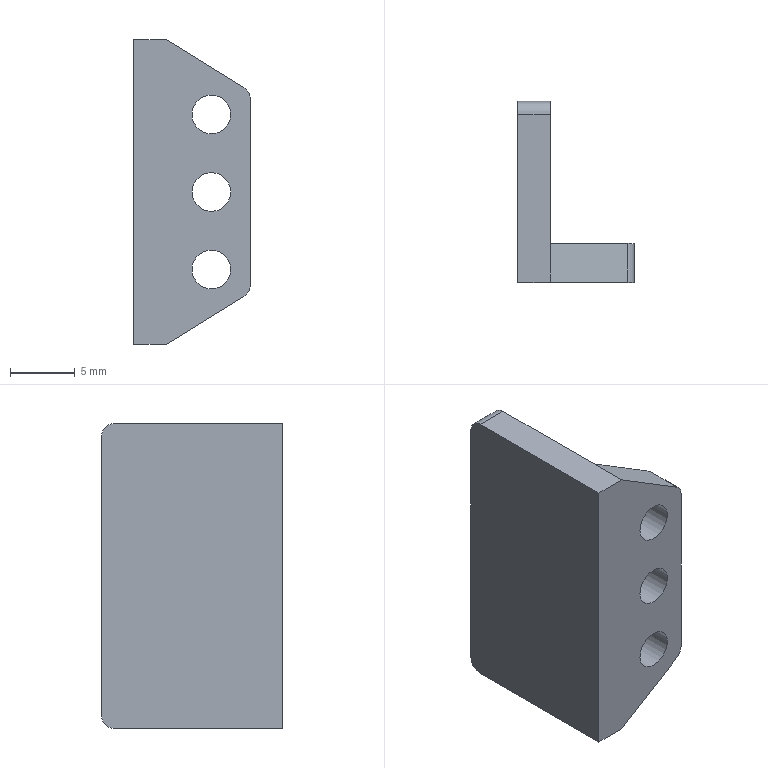Part | STEP file | 1-40.9 | 1 solid | 17 faces | box 9 x 14 x 23.6 mm | volume 1143 mm3 | plane 10 | cylinder 7 | commonest cylinder face diameters 2 x4 3 x3
STEP:
#1=CARTESIAN_POINT('',(0.,0.,0.));
#2=DIRECTION('',(0.,0.,1.));
#3=DIRECTION('',(1.,0.,0.));
#4=AXIS2_PLACEMENT_3D('',#1,#2,#3);
#5=CARTESIAN_POINT('',(5.,-7.,0.));
#6=VERTEX_POINT('',#5);
#7=CARTESIAN_POINT('',(3.5,-7.,0.));
#8=DIRECTION('',(0.,1.,0.));
#9=DIRECTION('',(1.,0.,0.));
#10=AXIS2_PLACEMENT_3D('',#7,#8,#9);
#11=CIRCLE('',#10,1.5);
#12=CARTESIAN_POINT('',(3.5,-7.,0.));
#13=DIRECTION('',(0.,1.,0.));
#14=DIRECTION('',(1.,0.,0.));
#15=AXIS2_PLACEMENT_3D('',#12,#13,#14);
#16=CYLINDRICAL_SURFACE('',#15,1.5);
#17=CARTESIAN_POINT('',(0.,0.));
#18=DIRECTION('',(1.,0.));
#19=VECTOR('',#18,1.);
#20=LINE('',#17,#19);
#21=(GEOMETRIC_REPRESENTATION_CONTEXT(2)PARAMETRIC_REPRESENTATION_CONTEXT()REPRESENTATION_CONTEXT('',''));
#22=DEFINITIONAL_REPRESENTATION('',(#20),#21);
#23=PCURVE('',#16,#22);
#24=CARTESIAN_POINT('',(11.14,-7.,0.));
#25=DIRECTION('',(0.,1.,0.));
#26=DIRECTION('',(0.,0.,-1.));
#27=AXIS2_PLACEMENT_3D('',#24,#25,#26);
#28=PLANE('',#27);
#29=CARTESIAN_POINT('',(0.,7.64));
#30=DIRECTION('',(0.,-1.));
#31=AXIS2_PLACEMENT_2D('',#29,#30);
#32=CIRCLE('',#31,1.5);
#33=(GEOMETRIC_REPRESENTATION_CONTEXT(2)PARAMETRIC_REPRESENTATION_CONTEXT()REPRESENTATION_CONTEXT('',''));
#34=DEFINITIONAL_REPRESENTATION('',(#32),#33);
#35=PCURVE('',#28,#34);
#36=SURFACE_CURVE('',#11,(#23,#35),.PCURVE_S1.);
#37=EDGE_CURVE('',#6,#6,#36,.T.);
#38=ORIENTED_EDGE('',*,*,#37,.T.);
#39=CARTESIAN_POINT('',(5.,-4.,0.));
#40=VERTEX_POINT('',#39);
#41=CARTESIAN_POINT('',(5.,-7.,0.));
#42=DIRECTION('',(0.,1.,0.));
#43=VECTOR('',#42,1.);
#44=LINE('',#41,#43);
#45=CARTESIAN_POINT('',(6.283,0.));
#46=DIRECTION('',(0.,1.));
#47=VECTOR('',#46,1.);
#48=LINE('',#45,#47);
#49=(GEOMETRIC_REPRESENTATION_CONTEXT(2)PARAMETRIC_REPRESENTATION_CONTEXT()REPRESENTATION_CONTEXT('',''));
#50=DEFINITIONAL_REPRESENTATION('',(#48),#49);
#51=PCURVE('',#16,#50);
#52=CARTESIAN_POINT('',(0.,0.));
#53=DIRECTION('',(0.,1.));
#54=VECTOR('',#53,1.);
#55=LINE('',#52,#54);
#56=(GEOMETRIC_REPRESENTATION_CONTEXT(2)PARAMETRIC_REPRESENTATION_CONTEXT()REPRESENTATION_CONTEXT('',''));
#57=DEFINITIONAL_REPRESENTATION('',(#55),#56);
#58=PCURVE('',#16,#57);
#59=SEAM_CURVE('',#44,(#51,#58),.PCURVE_S1.);
#60=EDGE_CURVE('',#6,#40,#59,.T.);
#61=ORIENTED_EDGE('',*,*,#60,.T.);
#62=CARTESIAN_POINT('',(3.5,-4.,0.));
#63=DIRECTION('',(0.,1.,0.));
#64=DIRECTION('',(1.,0.,0.));
#65=AXIS2_PLACEMENT_3D('',#62,#63,#64);
#66=CIRCLE('',#65,1.5);
#67=CARTESIAN_POINT('',(0.,3.));
#68=DIRECTION('',(1.,0.));
#69=VECTOR('',#68,1.);
#70=LINE('',#67,#69);
#71=(GEOMETRIC_REPRESENTATION_CONTEXT(2)PARAMETRIC_REPRESENTATION_CONTEXT()REPRESENTATION_CONTEXT('',''));
#72=DEFINITIONAL_REPRESENTATION('',(#70),#71);
#73=PCURVE('',#16,#72);
#74=CARTESIAN_POINT('',(11.8,-4.,0.));
#75=DIRECTION('',(0.,-1.,0.));
#76=DIRECTION('',(1.,0.,0.));
#77=AXIS2_PLACEMENT_3D('',#74,#75,#76);
#78=PLANE('',#77);
#79=CARTESIAN_POINT('',(-6.8,0.));
#80=CARTESIAN_POINT('',(-6.8,-2.598));
#81=CARTESIAN_POINT('',(-9.05,-1.299));
#82=CARTESIAN_POINT('',(-11.3,0.));
#83=CARTESIAN_POINT('',(-9.05,1.299));
#84=CARTESIAN_POINT('',(-6.8,2.598));
#85=CARTESIAN_POINT('',(-6.8,0.));
#86=(BOUNDED_CURVE()B_SPLINE_CURVE(2,(#79,#80,#81,#82,#83,#84,#85),.UNSPECIFIED.,.T.,.F.)B_SPLINE_CURVE_WITH_KNOTS((1,2,2,2,2,1),(-2.094,0.,2.094,4.189,6.283,8.378),.UNSPECIFIED.)CURVE()GEOMETRIC_REPRESENTATION_ITEM()RATIONAL_B_SPLINE_CURVE((1.,0.5,1.,0.5,1.,0.5,1.))REPRESENTATION_ITEM(''));
#87=(GEOMETRIC_REPRESENTATION_CONTEXT(2)PARAMETRIC_REPRESENTATION_CONTEXT()REPRESENTATION_CONTEXT('',''));
#88=DEFINITIONAL_REPRESENTATION('',(#86),#87);
#89=PCURVE('',#78,#88);
#90=SURFACE_CURVE('',#66,(#73,#89),.PCURVE_S1.);
#91=EDGE_CURVE('',#40,#40,#90,.T.);
#92=ORIENTED_EDGE('',*,*,#91,.F.);
#93=ORIENTED_EDGE('',*,*,#60,.F.);
#94=EDGE_LOOP('',(#38,#61,#92,#93));
#95=FACE_BOUND('',#94,.F.);
#96=ADVANCED_FACE('',(#95),#16,.F.);
#97=CARTESIAN_POINT('',(5.,-7.,6.));
#98=VERTEX_POINT('',#97);
#99=CARTESIAN_POINT('',(3.5,-7.,6.));
#100=DIRECTION('',(0.,1.,0.));
#101=DIRECTION('',(1.,0.,0.));
#102=AXIS2_PLACEMENT_3D('',#99,#100,#101);
#103=CIRCLE('',#102,1.5);
#104=CARTESIAN_POINT('',(3.5,-7.,6.));
#105=DIRECTION('',(0.,1.,0.));
#106=DIRECTION('',(1.,0.,0.));
#107=AXIS2_PLACEMENT_3D('',#104,#105,#106);
#108=CYLINDRICAL_SURFACE('',#107,1.5);
#109=CARTESIAN_POINT('',(0.,0.));
#110=DIRECTION('',(1.,0.));
#111=VECTOR('',#110,1.);
#112=LINE('',#109,#111);
#113=(GEOMETRIC_REPRESENTATION_CONTEXT(2)PARAMETRIC_REPRESENTATION_CONTEXT()REPRESENTATION_CONTEXT('',''));
#114=DEFINITIONAL_REPRESENTATION('',(#112),#113);
#115=PCURVE('',#108,#114);
#116=CARTESIAN_POINT('',(-6.,7.64));
#117=DIRECTION('',(0.,-1.));
#118=AXIS2_PLACEMENT_2D('',#116,#117);
#119=CIRCLE('',#118,1.5);
#120=(GEOMETRIC_REPRESENTATION_CONTEXT(2)PARAMETRIC_REPRESENTATION_CONTEXT()REPRESENTATION_CONTEXT('',''));
#121=DEFINITIONAL_REPRESENTATION('',(#119),#120);
#122=PCURVE('',#28,#121);
#123=SURFACE_CURVE('',#103,(#115,#122),.PCURVE_S1.);
#124=EDGE_CURVE('',#98,#98,#123,.T.);
#125=ORIENTED_EDGE('',*,*,#124,.T.);
#126=CARTESIAN_POINT('',(5.,-4.,6.));
#127=VERTEX_POINT('',#126);
#128=CARTESIAN_POINT('',(5.,-7.,6.));
#129=DIRECTION('',(0.,1.,0.));
#130=VECTOR('',#129,1.);
#131=LINE('',#128,#130);
#132=CARTESIAN_POINT('',(6.283,0.));
#133=DIRECTION('',(0.,1.));
#134=VECTOR('',#133,1.);
#135=LINE('',#132,#134);
#136=(GEOMETRIC_REPRESENTATION_CONTEXT(2)PARAMETRIC_REPRESENTATION_CONTEXT()REPRESENTATION_CONTEXT('',''));
#137=DEFINITIONAL_REPRESENTATION('',(#135),#136);
#138=PCURVE('',#108,#137);
#139=CARTESIAN_POINT('',(0.,0.));
#140=DIRECTION('',(0.,1.));
#141=VECTOR('',#140,1.);
#142=LINE('',#139,#141);
#143=(GEOMETRIC_REPRESENTATION_CONTEXT(2)PARAMETRIC_REPRESENTATION_CONTEXT()REPRESENTATION_CONTEXT('',''));
#144=DEFINITIONAL_REPRESENTATION('',(#142),#143);
#145=PCURVE('',#108,#144);
#146=SEAM_CURVE('',#131,(#138,#145),.PCURVE_S1.);
#147=EDGE_CURVE('',#98,#127,#146,.T.);
#148=ORIENTED_EDGE('',*,*,#147,.T.);
#149=CARTESIAN_POINT('',(3.5,-4.,6.));
#150=DIRECTION('',(0.,1.,0.));
#151=DIRECTION('',(1.,0.,0.));
#152=AXIS2_PLACEMENT_3D('',#149,#150,#151);
#153=CIRCLE('',#152,1.5);
#154=CARTESIAN_POINT('',(0.,3.));
#155=DIRECTION('',(1.,0.));
#156=VECTOR('',#155,1.);
#157=LINE('',#154,#156);
#158=(GEOMETRIC_REPRESENTATION_CONTEXT(2)PARAMETRIC_REPRESENTATION_CONTEXT()REPRESENTATION_CONTEXT('',''));
#159=DEFINITIONAL_REPRESENTATION('',(#157),#158);
#160=PCURVE('',#108,#159);
#161=CARTESIAN_POINT('',(-6.8,6.));
#162=CARTESIAN_POINT('',(-6.8,3.402));
#163=CARTESIAN_POINT('',(-9.05,4.701));
#164=CARTESIAN_POINT('',(-11.3,6.));
#165=CARTESIAN_POINT('',(-9.05,7.299));
#166=CARTESIAN_POINT('',(-6.8,8.598));
#167=CARTESIAN_POINT('',(-6.8,6.));
#168=(BOUNDED_CURVE()B_SPLINE_CURVE(2,(#161,#162,#163,#164,#165,#166,#167),.UNSPECIFIED.,.T.,.F.)B_SPLINE_CURVE_WITH_KNOTS((1,2,2,2,2,1),(-2.094,0.,2.094,4.189,6.283,8.378),.UNSPECIFIED.)CURVE()GEOMETRIC_REPRESENTATION_ITEM()RATIONAL_B_SPLINE_CURVE((1.,0.5,1.,0.5,1.,0.5,1.))REPRESENTATION_ITEM(''));
#169=(GEOMETRIC_REPRESENTATION_CONTEXT(2)PARAMETRIC_REPRESENTATION_CONTEXT()REPRESENTATION_CONTEXT('',''));
#170=DEFINITIONAL_REPRESENTATION('',(#168),#169);
#171=PCURVE('',#78,#170);
#172=SURFACE_CURVE('',#153,(#160,#171),.PCURVE_S1.);
#173=EDGE_CURVE('',#127,#127,#172,.T.);
#174=ORIENTED_EDGE('',*,*,#173,.F.);
#175=ORIENTED_EDGE('',*,*,#147,.F.);
#176=EDGE_LOOP('',(#125,#148,#174,#175));
#177=FACE_BOUND('',#176,.F.);
#178=ADVANCED_FACE('',(#177),#108,.F.);
#179=CARTESIAN_POINT('',(5.,-7.,-6.));
#180=VERTEX_POINT('',#179);
#181=CARTESIAN_POINT('',(3.5,-7.,-6.));
#182=DIRECTION('',(0.,1.,0.));
#183=DIRECTION('',(1.,0.,0.));
#184=AXIS2_PLACEMENT_3D('',#181,#182,#183);
#185=CIRCLE('',#184,1.5);
#186=CARTESIAN_POINT('',(3.5,-7.,-6.));
#187=DIRECTION('',(0.,1.,0.));
#188=DIRECTION('',(1.,0.,0.));
#189=AXIS2_PLACEMENT_3D('',#186,#187,#188);
#190=CYLINDRICAL_SURFACE('',#189,1.5);
#191=CARTESIAN_POINT('',(0.,0.));
#192=DIRECTION('',(1.,0.));
#193=VECTOR('',#192,1.);
#194=LINE('',#191,#193);
#195=(GEOMETRIC_REPRESENTATION_CONTEXT(2)PARAMETRIC_REPRESENTATION_CONTEXT()REPRESENTATION_CONTEXT('',''));
#196=DEFINITIONAL_REPRESENTATION('',(#194),#195);
#197=PCURVE('',#190,#196);
#198=CARTESIAN_POINT('',(6.,7.64));
#199=DIRECTION('',(0.,-1.));
#200=AXIS2_PLACEMENT_2D('',#198,#199);
#201=CIRCLE('',#200,1.5);
#202=(GEOMETRIC_REPRESENTATION_CONTEXT(2)PARAMETRIC_REPRESENTATION_CONTEXT()REPRESENTATION_CONTEXT('',''));
#203=DEFINITIONAL_REPRESENTATION('',(#201),#202);
#204=PCURVE('',#28,#203);
#205=SURFACE_CURVE('',#185,(#197,#204),.PCURVE_S1.);
#206=EDGE_CURVE('',#180,#180,#205,.T.);
#207=ORIENTED_EDGE('',*,*,#206,.T.);
#208=CARTESIAN_POINT('',(5.,-4.,-6.));
#209=VERTEX_POINT('',#208);
#210=CARTESIAN_POINT('',(5.,-7.,-6.));
#211=DIRECTION('',(0.,1.,0.));
#212=VECTOR('',#211,1.);
#213=LINE('',#210,#212);
#214=CARTESIAN_POINT('',(6.283,0.));
#215=DIRECTION('',(0.,1.));
#216=VECTOR('',#215,1.);
#217=LINE('',#214,#216);
#218=(GEOMETRIC_REPRESENTATION_CONTEXT(2)PARAMETRIC_REPRESENTATION_CONTEXT()REPRESENTATION_CONTEXT('',''));
#219=DEFINITIONAL_REPRESENTATION('',(#217),#218);
#220=PCURVE('',#190,#219);
#221=CARTESIAN_POINT('',(0.,0.));
#222=DIRECTION('',(0.,1.));
#223=VECTOR('',#222,1.);
#224=LINE('',#221,#223);
#225=(GEOMETRIC_REPRESENTATION_CONTEXT(2)PARAMETRIC_REPRESENTATION_CONTEXT()REPRESENTATION_CONTEXT('',''));
#226=DEFINITIONAL_REPRESENTATION('',(#224),#225);
#227=PCURVE('',#190,#226);
#228=SEAM_CURVE('',#213,(#220,#227),.PCURVE_S1.);
#229=EDGE_CURVE('',#180,#209,#228,.T.);
#230=ORIENTED_EDGE('',*,*,#229,.T.);
#231=CARTESIAN_POINT('',(3.5,-4.,-6.));
#232=DIRECTION('',(0.,1.,0.));
#233=DIRECTION('',(1.,0.,0.));
#234=AXIS2_PLACEMENT_3D('',#231,#232,#233);
#235=CIRCLE('',#234,1.5);
#236=CARTESIAN_POINT('',(0.,3.));
#237=DIRECTION('',(1.,0.));
#238=VECTOR('',#237,1.);
#239=LINE('',#236,#238);
#240=(GEOMETRIC_REPRESENTATION_CONTEXT(2)PARAMETRIC_REPRESENTATION_CONTEXT()REPRESENTATION_CONTEXT('',''));
#241=DEFINITIONAL_REPRESENTATION('',(#239),#240);
#242=PCURVE('',#190,#241);
#243=CARTESIAN_POINT('',(-6.8,-6.));
#244=CARTESIAN_POINT('',(-6.8,-8.598));
#245=CARTESIAN_POINT('',(-9.05,-7.299));
#246=CARTESIAN_POINT('',(-11.3,-6.));
#247=CARTESIAN_POINT('',(-9.05,-4.701));
#248=CARTESIAN_POINT('',(-6.8,-3.402));
#249=CARTESIAN_POINT('',(-6.8,-6.));
#250=(BOUNDED_CURVE()B_SPLINE_CURVE(2,(#243,#244,#245,#246,#247,#248,#249),.UNSPECIFIED.,.T.,.F.)B_SPLINE_CURVE_WITH_KNOTS((1,2,2,2,2,1),(-2.094,0.,2.094,4.189,6.283,8.378),.UNSPECIFIED.)CURVE()GEOMETRIC_REPRESENTATION_ITEM()RATIONAL_B_SPLINE_CURVE((1.,0.5,1.,0.5,1.,0.5,1.))REPRESENTATION_ITEM(''));
#251=(GEOMETRIC_REPRESENTATION_CONTEXT(2)PARAMETRIC_REPRESENTATION_CONTEXT()REPRESENTATION_CONTEXT('',''));
#252=DEFINITIONAL_REPRESENTATION('',(#250),#251);
#253=PCURVE('',#78,#252);
#254=SURFACE_CURVE('',#235,(#242,#253),.PCURVE_S1.);
#255=EDGE_CURVE('',#209,#209,#254,.T.);
#256=ORIENTED_EDGE('',*,*,#255,.F.);
#257=ORIENTED_EDGE('',*,*,#229,.F.);
#258=EDGE_LOOP('',(#207,#230,#256,#257));
#259=FACE_BOUND('',#258,.F.);
#260=ADVANCED_FACE('',(#259),#190,.F.);
#261=CARTESIAN_POINT('',(-2.5,-7.,-11.8));
#262=VERTEX_POINT('',#261);
#263=CARTESIAN_POINT('',(-2.5,6.,-11.8));
#264=VERTEX_POINT('',#263);
#265=CARTESIAN_POINT('',(-2.5,-7.,-11.8));
#266=DIRECTION('',(0.,1.,0.));
#267=VECTOR('',#266,1.);
#268=LINE('',#265,#267);
#269=CARTESIAN_POINT('',(-2.5,4.8,0.));
#270=DIRECTION('',(1.,0.,0.));
#271=DIRECTION('',(0.,1.,0.));
#272=AXIS2_PLACEMENT_3D('',#269,#270,#271);
#273=PLANE('',#272);
#274=CARTESIAN_POINT('',(-11.8,-11.8));
#275=DIRECTION('',(1.,0.));
#276=VECTOR('',#275,1.);
#277=LINE('',#274,#276);
#278=(GEOMETRIC_REPRESENTATION_CONTEXT(2)PARAMETRIC_REPRESENTATION_CONTEXT()REPRESENTATION_CONTEXT('',''));
#279=DEFINITIONAL_REPRESENTATION('',(#277),#278);
#280=PCURVE('',#273,#279);
#281=CARTESIAN_POINT('',(-1.25,0.,-11.8));
#282=DIRECTION('',(0.,0.,1.));
#283=DIRECTION('',(0.,1.,0.));
#284=AXIS2_PLACEMENT_3D('',#281,#282,#283);
#285=PLANE('',#284);
#286=CARTESIAN_POINT('',(-7.,1.25));
#287=DIRECTION('',(1.,0.));
#288=VECTOR('',#287,1.);
#289=LINE('',#286,#288);
#290=(GEOMETRIC_REPRESENTATION_CONTEXT(2)PARAMETRIC_REPRESENTATION_CONTEXT()REPRESENTATION_CONTEXT('',''));
#291=DEFINITIONAL_REPRESENTATION('',(#289),#290);
#292=PCURVE('',#285,#291);
#293=SURFACE_CURVE('',#268,(#280,#292),.PCURVE_S1.);
#294=EDGE_CURVE('',#262,#264,#293,.T.);
#295=ORIENTED_EDGE('',*,*,#294,.T.);
#296=CARTESIAN_POINT('',(-2.5,7.,-10.8));
#297=VERTEX_POINT('',#296);
#298=CARTESIAN_POINT('',(-2.5,6.,-10.8));
#299=DIRECTION('',(1.,0.,0.));
#300=DIRECTION('',(0.,0.,-1.));
#301=AXIS2_PLACEMENT_3D('',#298,#299,#300);
#302=CIRCLE('',#301,1.);
#303=CARTESIAN_POINT('',(1.2,-10.8));
#304=DIRECTION('',(0.,-1.));
#305=AXIS2_PLACEMENT_2D('',#303,#304);
#306=CIRCLE('',#305,1.);
#307=(GEOMETRIC_REPRESENTATION_CONTEXT(2)PARAMETRIC_REPRESENTATION_CONTEXT()REPRESENTATION_CONTEXT('',''));
#308=DEFINITIONAL_REPRESENTATION('',(#306),#307);
#309=PCURVE('',#273,#308);
#310=CARTESIAN_POINT('',(0.,6.,-10.8));
#311=DIRECTION('',(-1.,0.,0.));
#312=DIRECTION('',(0.,0.,-1.));
#313=AXIS2_PLACEMENT_3D('',#310,#311,#312);
#314=CYLINDRICAL_SURFACE('',#313,1.);
#315=CARTESIAN_POINT('',(6.283,2.5));
#316=DIRECTION('',(-1.,0.));
#317=VECTOR('',#316,1.);
#318=LINE('',#315,#317);
#319=(GEOMETRIC_REPRESENTATION_CONTEXT(2)PARAMETRIC_REPRESENTATION_CONTEXT()REPRESENTATION_CONTEXT('',''));
#320=DEFINITIONAL_REPRESENTATION('',(#318),#319);
#321=PCURVE('',#314,#320);
#322=SURFACE_CURVE('',#302,(#309,#321),.PCURVE_S1.);
#323=EDGE_CURVE('',#264,#297,#322,.T.);
#324=ORIENTED_EDGE('',*,*,#323,.T.);
#325=CARTESIAN_POINT('',(-2.5,7.,10.8));
#326=VERTEX_POINT('',#325);
#327=CARTESIAN_POINT('',(-2.5,7.,-10.8));
#328=DIRECTION('',(0.,0.,1.));
#329=VECTOR('',#328,1.);
#330=LINE('',#327,#329);
#331=CARTESIAN_POINT('',(2.2,-10.8));
#332=DIRECTION('',(0.,1.));
#333=VECTOR('',#332,1.);
#334=LINE('',#331,#333);
#335=(GEOMETRIC_REPRESENTATION_CONTEXT(2)PARAMETRIC_REPRESENTATION_CONTEXT()REPRESENTATION_CONTEXT('',''));
#336=DEFINITIONAL_REPRESENTATION('',(#334),#335);
#337=PCURVE('',#273,#336);
#338=CARTESIAN_POINT('',(-1.25,7.,0.));
#339=DIRECTION('',(0.,-1.,0.));
#340=DIRECTION('',(0.,0.,1.));
#341=AXIS2_PLACEMENT_3D('',#338,#339,#340);
#342=PLANE('',#341);
#343=CARTESIAN_POINT('',(-10.8,1.25));
#344=DIRECTION('',(1.,0.));
#345=VECTOR('',#344,1.);
#346=LINE('',#343,#345);
#347=(GEOMETRIC_REPRESENTATION_CONTEXT(2)PARAMETRIC_REPRESENTATION_CONTEXT()REPRESENTATION_CONTEXT('',''));
#348=DEFINITIONAL_REPRESENTATION('',(#346),#347);
#349=PCURVE('',#342,#348);
#350=SURFACE_CURVE('',#330,(#337,#349),.PCURVE_S1.);
#351=EDGE_CURVE('',#297,#326,#350,.T.);
#352=ORIENTED_EDGE('',*,*,#351,.T.);
#353=CARTESIAN_POINT('',(-2.5,6.,11.8));
#354=VERTEX_POINT('',#353);
#355=CARTESIAN_POINT('',(-2.5,6.,10.8));
#356=DIRECTION('',(1.,0.,0.));
#357=DIRECTION('',(0.,1.,0.));
#358=AXIS2_PLACEMENT_3D('',#355,#356,#357);
#359=CIRCLE('',#358,1.);
#360=CARTESIAN_POINT('',(1.2,10.8));
#361=DIRECTION('',(1.,0.));
#362=AXIS2_PLACEMENT_2D('',#360,#361);
#363=CIRCLE('',#362,1.);
#364=(GEOMETRIC_REPRESENTATION_CONTEXT(2)PARAMETRIC_REPRESENTATION_CONTEXT()REPRESENTATION_CONTEXT('',''));
#365=DEFINITIONAL_REPRESENTATION('',(#363),#364);
#366=PCURVE('',#273,#365);
#367=CARTESIAN_POINT('',(0.,6.,10.8));
#368=DIRECTION('',(-1.,0.,0.));
#369=DIRECTION('',(0.,1.,0.));
#370=AXIS2_PLACEMENT_3D('',#367,#368,#369);
#371=CYLINDRICAL_SURFACE('',#370,1.);
#372=CARTESIAN_POINT('',(6.283,2.5));
#373=DIRECTION('',(-1.,0.));
#374=VECTOR('',#373,1.);
#375=LINE('',#372,#374);
#376=(GEOMETRIC_REPRESENTATION_CONTEXT(2)PARAMETRIC_REPRESENTATION_CONTEXT()REPRESENTATION_CONTEXT('',''));
#377=DEFINITIONAL_REPRESENTATION('',(#375),#376);
#378=PCURVE('',#371,#377);
#379=SURFACE_CURVE('',#359,(#366,#378),.PCURVE_S1.);
#380=EDGE_CURVE('',#326,#354,#379,.T.);
#381=ORIENTED_EDGE('',*,*,#380,.T.);
#382=CARTESIAN_POINT('',(-2.5,-7.,11.8));
#383=VERTEX_POINT('',#382);
#384=CARTESIAN_POINT('',(-2.5,6.,11.8));
#385=DIRECTION('',(0.,-1.,0.));
#386=VECTOR('',#385,1.);
#387=LINE('',#384,#386);
#388=CARTESIAN_POINT('',(1.2,11.8));
#389=DIRECTION('',(-1.,0.));
#390=VECTOR('',#389,1.);
#391=LINE('',#388,#390);
#392=(GEOMETRIC_REPRESENTATION_CONTEXT(2)PARAMETRIC_REPRESENTATION_CONTEXT()REPRESENTATION_CONTEXT('',''));
#393=DEFINITIONAL_REPRESENTATION('',(#391),#392);
#394=PCURVE('',#273,#393);
#395=CARTESIAN_POINT('',(-1.25,0.,11.8));
#396=DIRECTION('',(0.,0.,-1.));
#397=DIRECTION('',(0.,-1.,0.));
#398=AXIS2_PLACEMENT_3D('',#395,#396,#397);
#399=PLANE('',#398);
#400=CARTESIAN_POINT('',(-6.,1.25));
#401=DIRECTION('',(1.,0.));
#402=VECTOR('',#401,1.);
#403=LINE('',#400,#402);
#404=(GEOMETRIC_REPRESENTATION_CONTEXT(2)PARAMETRIC_REPRESENTATION_CONTEXT()REPRESENTATION_CONTEXT('',''));
#405=DEFINITIONAL_REPRESENTATION('',(#403),#404);
#406=PCURVE('',#399,#405);
#407=SURFACE_CURVE('',#387,(#394,#406),.PCURVE_S1.);
#408=EDGE_CURVE('',#354,#383,#407,.T.);
#409=ORIENTED_EDGE('',*,*,#408,.T.);
#410=CARTESIAN_POINT('',(-2.5,-7.,11.8));
#411=DIRECTION('',(0.,0.,-1.));
#412=VECTOR('',#411,1.);
#413=LINE('',#410,#412);
#414=CARTESIAN_POINT('',(-11.8,11.8));
#415=DIRECTION('',(0.,-1.));
#416=VECTOR('',#415,1.);
#417=LINE('',#414,#416);
#418=(GEOMETRIC_REPRESENTATION_CONTEXT(2)PARAMETRIC_REPRESENTATION_CONTEXT()REPRESENTATION_CONTEXT('',''));
#419=DEFINITIONAL_REPRESENTATION('',(#417),#418);
#420=PCURVE('',#273,#419);
#421=CARTESIAN_POINT('',(-11.8,13.64));
#422=DIRECTION('',(1.,0.));
#423=VECTOR('',#422,1.);
#424=LINE('',#421,#423);
#425=(GEOMETRIC_REPRESENTATION_CONTEXT(2)PARAMETRIC_REPRESENTATION_CONTEXT()REPRESENTATION_CONTEXT('',''));
#426=DEFINITIONAL_REPRESENTATION('',(#424),#425);
#427=PCURVE('',#28,#426);
#428=SURFACE_CURVE('',#413,(#420,#427),.PCURVE_S1.);
#429=EDGE_CURVE('',#383,#262,#428,.T.);
#430=ORIENTED_EDGE('',*,*,#429,.T.);
#431=EDGE_LOOP('',(#295,#324,#352,#381,#409,#430));
#432=FACE_BOUND('',#431,.F.);
#433=ADVANCED_FACE('',(#432),#273,.F.);
#434=CARTESIAN_POINT('',(0.,-7.,-11.8));
#435=VERTEX_POINT('',#434);
#436=CARTESIAN_POINT('',(0.,-4.,-11.8));
#437=VERTEX_POINT('',#436);
#438=CARTESIAN_POINT('',(0.,-7.,-11.8));
#439=DIRECTION('',(0.,1.,0.));
#440=VECTOR('',#439,1.);
#441=LINE('',#438,#440);
#442=CARTESIAN_POINT('',(-7.,-1.25));
#443=DIRECTION('',(1.,0.));
#444=VECTOR('',#443,1.);
#445=LINE('',#442,#444);
#446=(GEOMETRIC_REPRESENTATION_CONTEXT(2)PARAMETRIC_REPRESENTATION_CONTEXT()REPRESENTATION_CONTEXT('',''));
#447=DEFINITIONAL_REPRESENTATION('',(#445),#446);
#448=PCURVE('',#285,#447);
#449=CARTESIAN_POINT('',(3.25,-5.5,-9.8));
#450=DIRECTION('',(-0.5241,0.,0.8517));
#451=DIRECTION('',(0.8517,0.,0.5241));
#452=AXIS2_PLACEMENT_3D('',#449,#450,#451);
#453=PLANE('',#452);
#454=CARTESIAN_POINT('',(-3.816,-1.5));
#455=DIRECTION('',(0.,1.));
#456=VECTOR('',#455,1.);
#457=LINE('',#454,#456);
#458=(GEOMETRIC_REPRESENTATION_CONTEXT(2)PARAMETRIC_REPRESENTATION_CONTEXT()REPRESENTATION_CONTEXT('',''));
#459=DEFINITIONAL_REPRESENTATION('',(#457),#458);
#460=PCURVE('',#453,#459);
#461=SURFACE_CURVE('',#441,(#448,#460),.PCURVE_S1.);
#462=EDGE_CURVE('',#435,#437,#461,.T.);
#463=ORIENTED_EDGE('',*,*,#462,.T.);
#464=CARTESIAN_POINT('',(0.,6.,-11.8));
#465=VERTEX_POINT('',#464);
#466=CARTESIAN_POINT('',(0.,-4.,-11.8));
#467=DIRECTION('',(0.,1.,0.));
#468=VECTOR('',#467,1.);
#469=LINE('',#466,#468);
#470=CARTESIAN_POINT('',(-4.,-1.25));
#471=DIRECTION('',(1.,0.));
#472=VECTOR('',#471,1.);
#473=LINE('',#470,#472);
#474=(GEOMETRIC_REPRESENTATION_CONTEXT(2)PARAMETRIC_REPRESENTATION_CONTEXT()REPRESENTATION_CONTEXT('',''));
#475=DEFINITIONAL_REPRESENTATION('',(#473),#474);
#476=PCURVE('',#285,#475);
#477=CARTESIAN_POINT('',(0.,4.8,0.));
#478=DIRECTION('',(1.,0.,0.));
#479=DIRECTION('',(0.,1.,0.));
#480=AXIS2_PLACEMENT_3D('',#477,#478,#479);
#481=PLANE('',#480);
#482=CARTESIAN_POINT('',(-8.8,-11.8));
#483=DIRECTION('',(1.,0.));
#484=VECTOR('',#483,1.);
#485=LINE('',#482,#484);
#486=(GEOMETRIC_REPRESENTATION_CONTEXT(2)PARAMETRIC_REPRESENTATION_CONTEXT()REPRESENTATION_CONTEXT('',''));
#487=DEFINITIONAL_REPRESENTATION('',(#485),#486);
#488=PCURVE('',#481,#487);
#489=SURFACE_CURVE('',#469,(#476,#488),.PCURVE_S1.);
#490=EDGE_CURVE('',#437,#465,#489,.T.);
#491=ORIENTED_EDGE('',*,*,#490,.T.);
#492=CARTESIAN_POINT('',(0.,6.,-11.8));
#493=DIRECTION('',(-1.,0.,0.));
#494=VECTOR('',#493,1.);
#495=LINE('',#492,#494);
#496=CARTESIAN_POINT('',(6.,-1.25));
#497=DIRECTION('',(0.,1.));
#498=VECTOR('',#497,1.);
#499=LINE('',#496,#498);
#500=(GEOMETRIC_REPRESENTATION_CONTEXT(2)PARAMETRIC_REPRESENTATION_CONTEXT()REPRESENTATION_CONTEXT('',''));
#501=DEFINITIONAL_REPRESENTATION('',(#499),#500);
#502=PCURVE('',#285,#501);
#503=CARTESIAN_POINT('',(6.283,0.));
#504=DIRECTION('',(0.,1.));
#505=VECTOR('',#504,1.);
#506=LINE('',#503,#505);
#507=(GEOMETRIC_REPRESENTATION_CONTEXT(2)PARAMETRIC_REPRESENTATION_CONTEXT()REPRESENTATION_CONTEXT('',''));
#508=DEFINITIONAL_REPRESENTATION('',(#506),#507);
#509=PCURVE('',#314,#508);
#510=SURFACE_CURVE('',#495,(#502,#509),.PCURVE_S1.);
#511=EDGE_CURVE('',#465,#264,#510,.T.);
#512=ORIENTED_EDGE('',*,*,#511,.T.);
#513=ORIENTED_EDGE('',*,*,#294,.F.);
#514=CARTESIAN_POINT('',(0.,-7.,-11.8));
#515=DIRECTION('',(-1.,0.,0.));
#516=VECTOR('',#515,1.);
#517=LINE('',#514,#516);
#518=CARTESIAN_POINT('',(-7.,-1.25));
#519=DIRECTION('',(0.,1.));
#520=VECTOR('',#519,1.);
#521=LINE('',#518,#520);
#522=(GEOMETRIC_REPRESENTATION_CONTEXT(2)PARAMETRIC_REPRESENTATION_CONTEXT()REPRESENTATION_CONTEXT('',''));
#523=DEFINITIONAL_REPRESENTATION('',(#521),#522);
#524=PCURVE('',#285,#523);
#525=CARTESIAN_POINT('',(11.8,11.14));
#526=DIRECTION('',(0.,1.));
#527=VECTOR('',#526,1.);
#528=LINE('',#525,#527);
#529=(GEOMETRIC_REPRESENTATION_CONTEXT(2)PARAMETRIC_REPRESENTATION_CONTEXT()REPRESENTATION_CONTEXT('',''));
#530=DEFINITIONAL_REPRESENTATION('',(#528),#529);
#531=PCURVE('',#28,#530);
#532=SURFACE_CURVE('',#517,(#524,#531),.PCURVE_S1.);
#533=EDGE_CURVE('',#435,#262,#532,.T.);
#534=ORIENTED_EDGE('',*,*,#533,.F.);
#535=EDGE_LOOP('',(#463,#491,#512,#513,#534));
#536=FACE_BOUND('',#535,.F.);
#537=ADVANCED_FACE('',(#536),#285,.F.);
#538=CARTESIAN_POINT('',(0.,7.,-10.8));
#539=VERTEX_POINT('',#538);
#540=CARTESIAN_POINT('',(0.,7.,10.8));
#541=VERTEX_POINT('',#540);
#542=CARTESIAN_POINT('',(0.,7.,-10.8));
#543=DIRECTION('',(0.,0.,1.));
#544=VECTOR('',#543,1.);
#545=LINE('',#542,#544);
#546=CARTESIAN_POINT('',(-10.8,-1.25));
#547=DIRECTION('',(1.,0.));
#548=VECTOR('',#547,1.);
#549=LINE('',#546,#548);
#550=(GEOMETRIC_REPRESENTATION_CONTEXT(2)PARAMETRIC_REPRESENTATION_CONTEXT()REPRESENTATION_CONTEXT('',''));
#551=DEFINITIONAL_REPRESENTATION('',(#549),#550);
#552=PCURVE('',#342,#551);
#553=CARTESIAN_POINT('',(2.2,-10.8));
#554=DIRECTION('',(0.,1.));
#555=VECTOR('',#554,1.);
#556=LINE('',#553,#555);
#557=(GEOMETRIC_REPRESENTATION_CONTEXT(2)PARAMETRIC_REPRESENTATION_CONTEXT()REPRESENTATION_CONTEXT('',''));
#558=DEFINITIONAL_REPRESENTATION('',(#556),#557);
#559=PCURVE('',#481,#558);
#560=SURFACE_CURVE('',#545,(#552,#559),.PCURVE_S1.);
#561=EDGE_CURVE('',#539,#541,#560,.T.);
#562=ORIENTED_EDGE('',*,*,#561,.T.);
#563=CARTESIAN_POINT('',(0.,7.,10.8));
#564=DIRECTION('',(-1.,0.,0.));
#565=VECTOR('',#564,1.);
#566=LINE('',#563,#565);
#567=CARTESIAN_POINT('',(10.8,-1.25));
#568=DIRECTION('',(0.,1.));
#569=VECTOR('',#568,1.);
#570=LINE('',#567,#569);
#571=(GEOMETRIC_REPRESENTATION_CONTEXT(2)PARAMETRIC_REPRESENTATION_CONTEXT()REPRESENTATION_CONTEXT('',''));
#572=DEFINITIONAL_REPRESENTATION('',(#570),#571);
#573=PCURVE('',#342,#572);
#574=CARTESIAN_POINT('',(6.283,0.));
#575=DIRECTION('',(0.,1.));
#576=VECTOR('',#575,1.);
#577=LINE('',#574,#576);
#578=(GEOMETRIC_REPRESENTATION_CONTEXT(2)PARAMETRIC_REPRESENTATION_CONTEXT()REPRESENTATION_CONTEXT('',''));
#579=DEFINITIONAL_REPRESENTATION('',(#577),#578);
#580=PCURVE('',#371,#579);
#581=SURFACE_CURVE('',#566,(#573,#580),.PCURVE_S1.);
#582=EDGE_CURVE('',#541,#326,#581,.T.);
#583=ORIENTED_EDGE('',*,*,#582,.T.);
#584=ORIENTED_EDGE('',*,*,#351,.F.);
#585=CARTESIAN_POINT('',(0.,7.,-10.8));
#586=DIRECTION('',(-1.,0.,0.));
#587=VECTOR('',#586,1.);
#588=LINE('',#585,#587);
#589=CARTESIAN_POINT('',(-10.8,-1.25));
#590=DIRECTION('',(0.,1.));
#591=VECTOR('',#590,1.);
#592=LINE('',#589,#591);
#593=(GEOMETRIC_REPRESENTATION_CONTEXT(2)PARAMETRIC_REPRESENTATION_CONTEXT()REPRESENTATION_CONTEXT('',''));
#594=DEFINITIONAL_REPRESENTATION('',(#592),#593);
#595=PCURVE('',#342,#594);
#596=CARTESIAN_POINT('',(4.712,0.));
#597=DIRECTION('',(0.,1.));
#598=VECTOR('',#597,1.);
#599=LINE('',#596,#598);
#600=(GEOMETRIC_REPRESENTATION_CONTEXT(2)PARAMETRIC_REPRESENTATION_CONTEXT()REPRESENTATION_CONTEXT('',''));
#601=DEFINITIONAL_REPRESENTATION('',(#599),#600);
#602=PCURVE('',#314,#601);
#603=SURFACE_CURVE('',#588,(#595,#602),.PCURVE_S1.);
#604=EDGE_CURVE('',#539,#297,#603,.T.);
#605=ORIENTED_EDGE('',*,*,#604,.F.);
#606=EDGE_LOOP('',(#562,#583,#584,#605));
#607=FACE_BOUND('',#606,.F.);
#608=ADVANCED_FACE('',(#607),#342,.F.);
#609=ORIENTED_EDGE('',*,*,#408,.F.);
#610=CARTESIAN_POINT('',(0.,6.,11.8));
#611=VERTEX_POINT('',#610);
#612=CARTESIAN_POINT('',(0.,6.,11.8));
#613=DIRECTION('',(-1.,0.,0.));
#614=VECTOR('',#613,1.);
#615=LINE('',#612,#614);
#616=CARTESIAN_POINT('',(-6.,-1.25));
#617=DIRECTION('',(0.,1.));
#618=VECTOR('',#617,1.);
#619=LINE('',#616,#618);
#620=(GEOMETRIC_REPRESENTATION_CONTEXT(2)PARAMETRIC_REPRESENTATION_CONTEXT()REPRESENTATION_CONTEXT('',''));
#621=DEFINITIONAL_REPRESENTATION('',(#619),#620);
#622=PCURVE('',#399,#621);
#623=CARTESIAN_POINT('',(4.712,0.));
#624=DIRECTION('',(0.,1.));
#625=VECTOR('',#624,1.);
#626=LINE('',#623,#625);
#627=(GEOMETRIC_REPRESENTATION_CONTEXT(2)PARAMETRIC_REPRESENTATION_CONTEXT()REPRESENTATION_CONTEXT('',''));
#628=DEFINITIONAL_REPRESENTATION('',(#626),#627);
#629=PCURVE('',#371,#628);
#630=SURFACE_CURVE('',#615,(#622,#629),.PCURVE_S1.);
#631=EDGE_CURVE('',#611,#354,#630,.T.);
#632=ORIENTED_EDGE('',*,*,#631,.F.);
#633=CARTESIAN_POINT('',(0.,-4.,11.8));
#634=VERTEX_POINT('',#633);
#635=CARTESIAN_POINT('',(0.,6.,11.8));
#636=DIRECTION('',(0.,-1.,0.));
#637=VECTOR('',#636,1.);
#638=LINE('',#635,#637);
#639=CARTESIAN_POINT('',(-6.,-1.25));
#640=DIRECTION('',(1.,0.));
#641=VECTOR('',#640,1.);
#642=LINE('',#639,#641);
#643=(GEOMETRIC_REPRESENTATION_CONTEXT(2)PARAMETRIC_REPRESENTATION_CONTEXT()REPRESENTATION_CONTEXT('',''));
#644=DEFINITIONAL_REPRESENTATION('',(#642),#643);
#645=PCURVE('',#399,#644);
#646=CARTESIAN_POINT('',(1.2,11.8));
#647=DIRECTION('',(-1.,0.));
#648=VECTOR('',#647,1.);
#649=LINE('',#646,#648);
#650=(GEOMETRIC_REPRESENTATION_CONTEXT(2)PARAMETRIC_REPRESENTATION_CONTEXT()REPRESENTATION_CONTEXT('',''));
#651=DEFINITIONAL_REPRESENTATION('',(#649),#650);
#652=PCURVE('',#481,#651);
#653=SURFACE_CURVE('',#638,(#645,#652),.PCURVE_S1.);
#654=EDGE_CURVE('',#611,#634,#653,.T.);
#655=ORIENTED_EDGE('',*,*,#654,.T.);
#656=CARTESIAN_POINT('',(0.,-7.,11.8));
#657=VERTEX_POINT('',#656);
#658=CARTESIAN_POINT('',(0.,-4.,11.8));
#659=DIRECTION('',(0.,-1.,0.));
#660=VECTOR('',#659,1.);
#661=LINE('',#658,#660);
#662=CARTESIAN_POINT('',(4.,-1.25));
#663=DIRECTION('',(1.,0.));
#664=VECTOR('',#663,1.);
#665=LINE('',#662,#664);
#666=(GEOMETRIC_REPRESENTATION_CONTEXT(2)PARAMETRIC_REPRESENTATION_CONTEXT()REPRESENTATION_CONTEXT('',''));
#667=DEFINITIONAL_REPRESENTATION('',(#665),#666);
#668=PCURVE('',#399,#667);
#669=CARTESIAN_POINT('',(3.25,-5.5,9.8));
#670=DIRECTION('',(-0.5241,0.,-0.8517));
#671=DIRECTION('',(-0.8517,0.,0.5241));
#672=AXIS2_PLACEMENT_3D('',#669,#670,#671);
#673=PLANE('',#672);
#674=CARTESIAN_POINT('',(3.816,1.5));
#675=DIRECTION('',(0.,-1.));
#676=VECTOR('',#675,1.);
#677=LINE('',#674,#676);
#678=(GEOMETRIC_REPRESENTATION_CONTEXT(2)PARAMETRIC_REPRESENTATION_CONTEXT()REPRESENTATION_CONTEXT('',''));
#679=DEFINITIONAL_REPRESENTATION('',(#677),#678);
#680=PCURVE('',#673,#679);
#681=SURFACE_CURVE('',#661,(#668,#680),.PCURVE_S1.);
#682=EDGE_CURVE('',#634,#657,#681,.T.);
#683=ORIENTED_EDGE('',*,*,#682,.T.);
#684=CARTESIAN_POINT('',(0.,-7.,11.8));
#685=DIRECTION('',(-1.,0.,0.));
#686=VECTOR('',#685,1.);
#687=LINE('',#684,#686);
#688=CARTESIAN_POINT('',(7.,-1.25));
#689=DIRECTION('',(0.,1.));
#690=VECTOR('',#689,1.);
#691=LINE('',#688,#690);
#692=(GEOMETRIC_REPRESENTATION_CONTEXT(2)PARAMETRIC_REPRESENTATION_CONTEXT()REPRESENTATION_CONTEXT('',''));
#693=DEFINITIONAL_REPRESENTATION('',(#691),#692);
#694=PCURVE('',#399,#693);
#695=CARTESIAN_POINT('',(-11.8,11.14));
#696=DIRECTION('',(0.,1.));
#697=VECTOR('',#696,1.);
#698=LINE('',#695,#697);
#699=(GEOMETRIC_REPRESENTATION_CONTEXT(2)PARAMETRIC_REPRESENTATION_CONTEXT()REPRESENTATION_CONTEXT('',''));
#700=DEFINITIONAL_REPRESENTATION('',(#698),#699);
#701=PCURVE('',#28,#700);
#702=SURFACE_CURVE('',#687,(#694,#701),.PCURVE_S1.);
#703=EDGE_CURVE('',#657,#383,#702,.T.);
#704=ORIENTED_EDGE('',*,*,#703,.T.);
#705=EDGE_LOOP('',(#609,#632,#655,#683,#704));
#706=FACE_BOUND('',#705,.F.);
#707=ADVANCED_FACE('',(#706),#399,.F.);
#708=CARTESIAN_POINT('',(0.,-4.,11.8));
#709=DIRECTION('',(0.,0.,-1.));
#710=VECTOR('',#709,1.);
#711=LINE('',#708,#710);
#712=CARTESIAN_POINT('',(-8.8,11.8));
#713=DIRECTION('',(0.,-1.));
#714=VECTOR('',#713,1.);
#715=LINE('',#712,#714);
#716=(GEOMETRIC_REPRESENTATION_CONTEXT(2)PARAMETRIC_REPRESENTATION_CONTEXT()REPRESENTATION_CONTEXT('',''));
#717=DEFINITIONAL_REPRESENTATION('',(#715),#716);
#718=PCURVE('',#481,#717);
#719=CARTESIAN_POINT('',(-11.8,11.8));
#720=DIRECTION('',(0.,-1.));
#721=VECTOR('',#720,1.);
#722=LINE('',#719,#721);
#723=(GEOMETRIC_REPRESENTATION_CONTEXT(2)PARAMETRIC_REPRESENTATION_CONTEXT()REPRESENTATION_CONTEXT('',''));
#724=DEFINITIONAL_REPRESENTATION('',(#722),#723);
#725=PCURVE('',#78,#724);
#726=SURFACE_CURVE('',#711,(#718,#725),.PCURVE_S1.);
#727=EDGE_CURVE('',#634,#437,#726,.T.);
#728=ORIENTED_EDGE('',*,*,#727,.T.);
#729=ORIENTED_EDGE('',*,*,#490,.T.);
#730=CARTESIAN_POINT('',(0.,6.,-10.8));
#731=DIRECTION('',(1.,0.,0.));
#732=DIRECTION('',(0.,0.,-1.));
#733=AXIS2_PLACEMENT_3D('',#730,#731,#732);
#734=CIRCLE('',#733,1.);
#735=CARTESIAN_POINT('',(1.2,-10.8));
#736=DIRECTION('',(0.,-1.));
#737=AXIS2_PLACEMENT_2D('',#735,#736);
#738=CIRCLE('',#737,1.);
#739=(GEOMETRIC_REPRESENTATION_CONTEXT(2)PARAMETRIC_REPRESENTATION_CONTEXT()REPRESENTATION_CONTEXT('',''));
#740=DEFINITIONAL_REPRESENTATION('',(#738),#739);
#741=PCURVE('',#481,#740);
#742=CARTESIAN_POINT('',(6.283,0.));
#743=DIRECTION('',(-1.,0.));
#744=VECTOR('',#743,1.);
#745=LINE('',#742,#744);
#746=(GEOMETRIC_REPRESENTATION_CONTEXT(2)PARAMETRIC_REPRESENTATION_CONTEXT()REPRESENTATION_CONTEXT('',''));
#747=DEFINITIONAL_REPRESENTATION('',(#745),#746);
#748=PCURVE('',#314,#747);
#749=SURFACE_CURVE('',#734,(#741,#748),.PCURVE_S1.);
#750=EDGE_CURVE('',#465,#539,#749,.T.);
#751=ORIENTED_EDGE('',*,*,#750,.T.);
#752=ORIENTED_EDGE('',*,*,#561,.T.);
#753=CARTESIAN_POINT('',(0.,6.,10.8));
#754=DIRECTION('',(1.,0.,0.));
#755=DIRECTION('',(0.,1.,0.));
#756=AXIS2_PLACEMENT_3D('',#753,#754,#755);
#757=CIRCLE('',#756,1.);
#758=CARTESIAN_POINT('',(1.2,10.8));
#759=DIRECTION('',(1.,0.));
#760=AXIS2_PLACEMENT_2D('',#758,#759);
#761=CIRCLE('',#760,1.);
#762=(GEOMETRIC_REPRESENTATION_CONTEXT(2)PARAMETRIC_REPRESENTATION_CONTEXT()REPRESENTATION_CONTEXT('',''));
#763=DEFINITIONAL_REPRESENTATION('',(#761),#762);
#764=PCURVE('',#481,#763);
#765=CARTESIAN_POINT('',(6.283,0.));
#766=DIRECTION('',(-1.,0.));
#767=VECTOR('',#766,1.);
#768=LINE('',#765,#767);
#769=(GEOMETRIC_REPRESENTATION_CONTEXT(2)PARAMETRIC_REPRESENTATION_CONTEXT()REPRESENTATION_CONTEXT('',''));
#770=DEFINITIONAL_REPRESENTATION('',(#768),#769);
#771=PCURVE('',#371,#770);
#772=SURFACE_CURVE('',#757,(#764,#771),.PCURVE_S1.);
#773=EDGE_CURVE('',#541,#611,#772,.T.);
#774=ORIENTED_EDGE('',*,*,#773,.T.);
#775=ORIENTED_EDGE('',*,*,#654,.T.);
#776=EDGE_LOOP('',(#728,#729,#751,#752,#774,#775));
#777=FACE_BOUND('',#776,.T.);
#778=ADVANCED_FACE('',(#777),#481,.T.);
#779=ORIENTED_EDGE('',*,*,#511,.T.);
#780=ORIENTED_EDGE('',*,*,#323,.T.);
#781=ORIENTED_EDGE('',*,*,#604,.F.);
#782=ORIENTED_EDGE('',*,*,#750,.F.);
#783=EDGE_LOOP('',(#779,#780,#781,#782));
#784=FACE_BOUND('',#783,.T.);
#785=ADVANCED_FACE('',(#784),#314,.T.);
#786=ORIENTED_EDGE('',*,*,#582,.T.);
#787=ORIENTED_EDGE('',*,*,#380,.T.);
#788=ORIENTED_EDGE('',*,*,#631,.F.);
#789=ORIENTED_EDGE('',*,*,#773,.F.);
#790=EDGE_LOOP('',(#786,#787,#788,#789));
#791=FACE_BOUND('',#790,.T.);
#792=ADVANCED_FACE('',(#791),#371,.T.);
#793=ORIENTED_EDGE('',*,*,#533,.T.);
#794=ORIENTED_EDGE('',*,*,#429,.F.);
#795=ORIENTED_EDGE('',*,*,#703,.F.);
#796=CARTESIAN_POINT('',(6.024,-7.,8.093));
#797=VERTEX_POINT('',#796);
#798=CARTESIAN_POINT('',(6.024,-7.,8.093));
#799=DIRECTION('',(-0.8517,0.,0.5241));
#800=VECTOR('',#799,1.);
#801=LINE('',#798,#800);
#802=CARTESIAN_POINT('',(-8.093,5.116));
#803=DIRECTION('',(-0.5241,0.8517));
#804=VECTOR('',#803,1.);
#805=LINE('',#802,#804);
#806=(GEOMETRIC_REPRESENTATION_CONTEXT(2)PARAMETRIC_REPRESENTATION_CONTEXT()REPRESENTATION_CONTEXT('',''));
#807=DEFINITIONAL_REPRESENTATION('',(#805),#806);
#808=PCURVE('',#28,#807);
#809=CARTESIAN_POINT('',(-3.257,-1.5));
#810=DIRECTION('',(1.,0.));
#811=VECTOR('',#810,1.);
#812=LINE('',#809,#811);
#813=(GEOMETRIC_REPRESENTATION_CONTEXT(2)PARAMETRIC_REPRESENTATION_CONTEXT()REPRESENTATION_CONTEXT('',''));
#814=DEFINITIONAL_REPRESENTATION('',(#812),#813);
#815=PCURVE('',#673,#814);
#816=SURFACE_CURVE('',#801,(#808,#815),.PCURVE_S1.);
#817=EDGE_CURVE('',#797,#657,#816,.T.);
#818=ORIENTED_EDGE('',*,*,#817,.F.);
#819=CARTESIAN_POINT('',(6.5,-7.,7.241));
#820=VERTEX_POINT('',#819);
#821=CARTESIAN_POINT('',(5.5,-7.,7.241));
#822=DIRECTION('',(0.,-1.,0.));
#823=DIRECTION('',(1.,0.,0.));
#824=AXIS2_PLACEMENT_3D('',#821,#822,#823);
#825=CIRCLE('',#824,1.);
#826=CARTESIAN_POINT('',(-7.241,4.64));
#827=CARTESIAN_POINT('',(-8.973,4.64));
#828=CARTESIAN_POINT('',(-8.107,6.14));
#829=CARTESIAN_POINT('',(-7.241,7.64));
#830=CARTESIAN_POINT('',(-6.375,6.14));
#831=CARTESIAN_POINT('',(-5.509,4.64));
#832=CARTESIAN_POINT('',(-7.241,4.64));
#833=(BOUNDED_CURVE()B_SPLINE_CURVE(2,(#826,#827,#828,#829,#830,#831,#832),.UNSPECIFIED.,.T.,.F.)B_SPLINE_CURVE_WITH_KNOTS((1,2,2,2,2,1),(-2.094,0.,2.094,4.189,6.283,8.378),.UNSPECIFIED.)CURVE()GEOMETRIC_REPRESENTATION_ITEM()RATIONAL_B_SPLINE_CURVE((1.,0.5,1.,0.5,1.,0.5,1.))REPRESENTATION_ITEM(''));
#834=(GEOMETRIC_REPRESENTATION_CONTEXT(2)PARAMETRIC_REPRESENTATION_CONTEXT()REPRESENTATION_CONTEXT('',''));
#835=DEFINITIONAL_REPRESENTATION('',(#833),#834);
#836=PCURVE('',#28,#835);
#837=CARTESIAN_POINT('',(5.5,-7.,7.241));
#838=DIRECTION('',(0.,1.,0.));
#839=DIRECTION('',(1.,0.,0.));
#840=AXIS2_PLACEMENT_3D('',#837,#838,#839);
#841=CYLINDRICAL_SURFACE('',#840,1.);
#842=CARTESIAN_POINT('',(6.283,0.));
#843=DIRECTION('',(-1.,0.));
#844=VECTOR('',#843,1.);
#845=LINE('',#842,#844);
#846=(GEOMETRIC_REPRESENTATION_CONTEXT(2)PARAMETRIC_REPRESENTATION_CONTEXT()REPRESENTATION_CONTEXT('',''));
#847=DEFINITIONAL_REPRESENTATION('',(#845),#846);
#848=PCURVE('',#841,#847);
#849=SURFACE_CURVE('',#825,(#836,#848),.PCURVE_S1.);
#850=EDGE_CURVE('',#820,#797,#849,.T.);
#851=ORIENTED_EDGE('',*,*,#850,.F.);
#852=CARTESIAN_POINT('',(6.5,-7.,-7.241));
#853=VERTEX_POINT('',#852);
#854=CARTESIAN_POINT('',(6.5,-7.,-7.241));
#855=DIRECTION('',(0.,0.,1.));
#856=VECTOR('',#855,1.);
#857=LINE('',#854,#856);
#858=CARTESIAN_POINT('',(7.241,4.64));
#859=DIRECTION('',(-1.,0.));
#860=VECTOR('',#859,1.);
#861=LINE('',#858,#860);
#862=(GEOMETRIC_REPRESENTATION_CONTEXT(2)PARAMETRIC_REPRESENTATION_CONTEXT()REPRESENTATION_CONTEXT('',''));
#863=DEFINITIONAL_REPRESENTATION('',(#861),#862);
#864=PCURVE('',#28,#863);
#865=CARTESIAN_POINT('',(6.5,-5.5,0.));
#866=DIRECTION('',(-1.,0.,0.));
#867=DIRECTION('',(0.,0.,1.));
#868=AXIS2_PLACEMENT_3D('',#865,#866,#867);
#869=PLANE('',#868);
#870=CARTESIAN_POINT('',(-7.241,-1.5));
#871=DIRECTION('',(1.,0.));
#872=VECTOR('',#871,1.);
#873=LINE('',#870,#872);
#874=(GEOMETRIC_REPRESENTATION_CONTEXT(2)PARAMETRIC_REPRESENTATION_CONTEXT()REPRESENTATION_CONTEXT('',''));
#875=DEFINITIONAL_REPRESENTATION('',(#873),#874);
#876=PCURVE('',#869,#875);
#877=SURFACE_CURVE('',#857,(#864,#876),.PCURVE_S1.);
#878=EDGE_CURVE('',#853,#820,#877,.T.);
#879=ORIENTED_EDGE('',*,*,#878,.F.);
#880=CARTESIAN_POINT('',(6.024,-7.,-8.093));
#881=VERTEX_POINT('',#880);
#882=CARTESIAN_POINT('',(5.5,-7.,-7.241));
#883=DIRECTION('',(0.,-1.,0.));
#884=DIRECTION('',(0.5241,0.,-0.8517));
#885=AXIS2_PLACEMENT_3D('',#882,#883,#884);
#886=CIRCLE('',#885,1.);
#887=CARTESIAN_POINT('',(8.093,5.116));
#888=CARTESIAN_POINT('',(7.185,3.641));
#889=CARTESIAN_POINT('',(6.361,5.164));
#890=CARTESIAN_POINT('',(5.538,6.688));
#891=CARTESIAN_POINT('',(7.269,6.64));
#892=CARTESIAN_POINT('',(9.001,6.591));
#893=CARTESIAN_POINT('',(8.093,5.116));
#894=(BOUNDED_CURVE()B_SPLINE_CURVE(2,(#887,#888,#889,#890,#891,#892,#893),.UNSPECIFIED.,.T.,.F.)B_SPLINE_CURVE_WITH_KNOTS((1,2,2,2,2,1),(-2.094,0.,2.094,4.189,6.283,8.378),.UNSPECIFIED.)CURVE()GEOMETRIC_REPRESENTATION_ITEM()RATIONAL_B_SPLINE_CURVE((1.,0.5,1.,0.5,1.,0.5,1.))REPRESENTATION_ITEM(''));
#895=(GEOMETRIC_REPRESENTATION_CONTEXT(2)PARAMETRIC_REPRESENTATION_CONTEXT()REPRESENTATION_CONTEXT('',''));
#896=DEFINITIONAL_REPRESENTATION('',(#894),#895);
#897=PCURVE('',#28,#896);
#898=CARTESIAN_POINT('',(5.5,-7.,-7.241));
#899=DIRECTION('',(0.,1.,0.));
#900=DIRECTION('',(0.5241,0.,-0.8517));
#901=AXIS2_PLACEMENT_3D('',#898,#899,#900);
#902=CYLINDRICAL_SURFACE('',#901,1.);
#903=CARTESIAN_POINT('',(6.283,0.));
#904=DIRECTION('',(-1.,0.));
#905=VECTOR('',#904,1.);
#906=LINE('',#903,#905);
#907=(GEOMETRIC_REPRESENTATION_CONTEXT(2)PARAMETRIC_REPRESENTATION_CONTEXT()REPRESENTATION_CONTEXT('',''));
#908=DEFINITIONAL_REPRESENTATION('',(#906),#907);
#909=PCURVE('',#902,#908);
#910=SURFACE_CURVE('',#886,(#897,#909),.PCURVE_S1.);
#911=EDGE_CURVE('',#881,#853,#910,.T.);
#912=ORIENTED_EDGE('',*,*,#911,.F.);
#913=CARTESIAN_POINT('',(0.,-7.,-11.8));
#914=DIRECTION('',(0.8517,0.,0.5241));
#915=VECTOR('',#914,1.);
#916=LINE('',#913,#915);
#917=CARTESIAN_POINT('',(11.8,11.14));
#918=DIRECTION('',(-0.5241,-0.8517));
#919=VECTOR('',#918,1.);
#920=LINE('',#917,#919);
#921=(GEOMETRIC_REPRESENTATION_CONTEXT(2)PARAMETRIC_REPRESENTATION_CONTEXT()REPRESENTATION_CONTEXT('',''));
#922=DEFINITIONAL_REPRESENTATION('',(#920),#921);
#923=PCURVE('',#28,#922);
#924=CARTESIAN_POINT('',(-3.816,-1.5));
#925=DIRECTION('',(1.,0.));
#926=VECTOR('',#925,1.);
#927=LINE('',#924,#926);
#928=(GEOMETRIC_REPRESENTATION_CONTEXT(2)PARAMETRIC_REPRESENTATION_CONTEXT()REPRESENTATION_CONTEXT('',''));
#929=DEFINITIONAL_REPRESENTATION('',(#927),#928);
#930=PCURVE('',#453,#929);
#931=SURFACE_CURVE('',#916,(#923,#930),.PCURVE_S1.);
#932=EDGE_CURVE('',#435,#881,#931,.T.);
#933=ORIENTED_EDGE('',*,*,#932,.F.);
#934=EDGE_LOOP('',(#793,#794,#795,#818,#851,#879,#912,#933));
#935=FACE_BOUND('',#934,.F.);
#936=ORIENTED_EDGE('',*,*,#37,.F.);
#937=EDGE_LOOP('',(#936));
#938=FACE_BOUND('',#937,.F.);
#939=ORIENTED_EDGE('',*,*,#124,.F.);
#940=EDGE_LOOP('',(#939));
#941=FACE_BOUND('',#940,.F.);
#942=ORIENTED_EDGE('',*,*,#206,.F.);
#943=EDGE_LOOP('',(#942));
#944=FACE_BOUND('',#943,.F.);
#945=ADVANCED_FACE('',(#935,#938,#941,#944),#28,.F.);
#946=ORIENTED_EDGE('',*,*,#932,.T.);
#947=CARTESIAN_POINT('',(6.024,-4.,-8.093));
#948=VERTEX_POINT('',#947);
#949=CARTESIAN_POINT('',(6.024,-7.,-8.093));
#950=DIRECTION('',(0.,1.,0.));
#951=VECTOR('',#950,1.);
#952=LINE('',#949,#951);
#953=CARTESIAN_POINT('',(3.257,-1.5));
#954=DIRECTION('',(0.,1.));
#955=VECTOR('',#954,1.);
#956=LINE('',#953,#955);
#957=(GEOMETRIC_REPRESENTATION_CONTEXT(2)PARAMETRIC_REPRESENTATION_CONTEXT()REPRESENTATION_CONTEXT('',''));
#958=DEFINITIONAL_REPRESENTATION('',(#956),#957);
#959=PCURVE('',#453,#958);
#960=CARTESIAN_POINT('',(6.283,0.));
#961=DIRECTION('',(0.,1.));
#962=VECTOR('',#961,1.);
#963=LINE('',#960,#962);
#964=(GEOMETRIC_REPRESENTATION_CONTEXT(2)PARAMETRIC_REPRESENTATION_CONTEXT()REPRESENTATION_CONTEXT('',''));
#965=DEFINITIONAL_REPRESENTATION('',(#963),#964);
#966=PCURVE('',#902,#965);
#967=SURFACE_CURVE('',#952,(#959,#966),.PCURVE_S1.);
#968=EDGE_CURVE('',#881,#948,#967,.T.);
#969=ORIENTED_EDGE('',*,*,#968,.T.);
#970=CARTESIAN_POINT('',(0.,-4.,-11.8));
#971=DIRECTION('',(0.8517,0.,0.5241));
#972=VECTOR('',#971,1.);
#973=LINE('',#970,#972);
#974=CARTESIAN_POINT('',(-3.816,1.5));
#975=DIRECTION('',(1.,0.));
#976=VECTOR('',#975,1.);
#977=LINE('',#974,#976);
#978=(GEOMETRIC_REPRESENTATION_CONTEXT(2)PARAMETRIC_REPRESENTATION_CONTEXT()REPRESENTATION_CONTEXT('',''));
#979=DEFINITIONAL_REPRESENTATION('',(#977),#978);
#980=PCURVE('',#453,#979);
#981=CARTESIAN_POINT('',(-11.8,-11.8));
#982=DIRECTION('',(0.8517,0.5241));
#983=VECTOR('',#982,1.);
#984=LINE('',#981,#983);
#985=(GEOMETRIC_REPRESENTATION_CONTEXT(2)PARAMETRIC_REPRESENTATION_CONTEXT()REPRESENTATION_CONTEXT('',''));
#986=DEFINITIONAL_REPRESENTATION('',(#984),#985);
#987=PCURVE('',#78,#986);
#988=SURFACE_CURVE('',#973,(#980,#987),.PCURVE_S1.);
#989=EDGE_CURVE('',#437,#948,#988,.T.);
#990=ORIENTED_EDGE('',*,*,#989,.F.);
#991=ORIENTED_EDGE('',*,*,#462,.F.);
#992=EDGE_LOOP('',(#946,#969,#990,#991));
#993=FACE_BOUND('',#992,.F.);
#994=ADVANCED_FACE('',(#993),#453,.F.);
#995=CARTESIAN_POINT('',(6.024,-4.,8.093));
#996=VERTEX_POINT('',#995);
#997=CARTESIAN_POINT('',(6.024,-4.,8.093));
#998=DIRECTION('',(-0.8517,0.,0.5241));
#999=VECTOR('',#998,1.);
#1000=LINE('',#997,#999);
#1001=CARTESIAN_POINT('',(-3.257,1.5));
#1002=DIRECTION('',(1.,0.));
#1003=VECTOR('',#1002,1.);
#1004=LINE('',#1001,#1003);
#1005=(GEOMETRIC_REPRESENTATION_CONTEXT(2)PARAMETRIC_REPRESENTATION_CONTEXT()REPRESENTATION_CONTEXT('',''));
#1006=DEFINITIONAL_REPRESENTATION('',(#1004),#1005);
#1007=PCURVE('',#673,#1006);
#1008=CARTESIAN_POINT('',(-5.776,8.093));
#1009=DIRECTION('',(-0.8517,0.5241));
#1010=VECTOR('',#1009,1.);
#1011=LINE('',#1008,#1010);
#1012=(GEOMETRIC_REPRESENTATION_CONTEXT(2)PARAMETRIC_REPRESENTATION_CONTEXT()REPRESENTATION_CONTEXT('',''));
#1013=DEFINITIONAL_REPRESENTATION('',(#1011),#1012);
#1014=PCURVE('',#78,#1013);
#1015=SURFACE_CURVE('',#1000,(#1007,#1014),.PCURVE_S1.);
#1016=EDGE_CURVE('',#996,#634,#1015,.T.);
#1017=ORIENTED_EDGE('',*,*,#1016,.F.);
#1018=CARTESIAN_POINT('',(6.024,-7.,8.093));
#1019=DIRECTION('',(0.,1.,0.));
#1020=VECTOR('',#1019,1.);
#1021=LINE('',#1018,#1020);
#1022=CARTESIAN_POINT('',(-3.257,-1.5));
#1023=DIRECTION('',(0.,1.));
#1024=VECTOR('',#1023,1.);
#1025=LINE('',#1022,#1024);
#1026=(GEOMETRIC_REPRESENTATION_CONTEXT(2)PARAMETRIC_REPRESENTATION_CONTEXT()REPRESENTATION_CONTEXT('',''));
#1027=DEFINITIONAL_REPRESENTATION('',(#1025),#1026);
#1028=PCURVE('',#673,#1027);
#1029=CARTESIAN_POINT('',(5.264,0.));
#1030=DIRECTION('',(0.,1.));
#1031=VECTOR('',#1030,1.);
#1032=LINE('',#1029,#1031);
#1033=(GEOMETRIC_REPRESENTATION_CONTEXT(2)PARAMETRIC_REPRESENTATION_CONTEXT()REPRESENTATION_CONTEXT('',''));
#1034=DEFINITIONAL_REPRESENTATION('',(#1032),#1033);
#1035=PCURVE('',#841,#1034);
#1036=SURFACE_CURVE('',#1021,(#1028,#1035),.PCURVE_S1.);
#1037=EDGE_CURVE('',#797,#996,#1036,.T.);
#1038=ORIENTED_EDGE('',*,*,#1037,.F.);
#1039=ORIENTED_EDGE('',*,*,#817,.T.);
#1040=ORIENTED_EDGE('',*,*,#682,.F.);
#1041=EDGE_LOOP('',(#1017,#1038,#1039,#1040));
#1042=FACE_BOUND('',#1041,.F.);
#1043=ADVANCED_FACE('',(#1042),#673,.F.);
#1044=ORIENTED_EDGE('',*,*,#989,.T.);
#1045=CARTESIAN_POINT('',(6.5,-4.,-7.241));
#1046=VERTEX_POINT('',#1045);
#1047=CARTESIAN_POINT('',(5.5,-4.,-7.241));
#1048=DIRECTION('',(0.,-1.,0.));
#1049=DIRECTION('',(0.5241,0.,-0.8517));
#1050=AXIS2_PLACEMENT_3D('',#1047,#1048,#1049);
#1051=CIRCLE('',#1050,1.);
#1052=CARTESIAN_POINT('',(-6.3,-7.241));
#1053=DIRECTION('',(0.5241,-0.8517));
#1054=AXIS2_PLACEMENT_2D('',#1052,#1053);
#1055=CIRCLE('',#1054,1.);
#1056=(GEOMETRIC_REPRESENTATION_CONTEXT(2)PARAMETRIC_REPRESENTATION_CONTEXT()REPRESENTATION_CONTEXT('',''));
#1057=DEFINITIONAL_REPRESENTATION('',(#1055),#1056);
#1058=PCURVE('',#78,#1057);
#1059=CARTESIAN_POINT('',(6.283,3.));
#1060=DIRECTION('',(-1.,0.));
#1061=VECTOR('',#1060,1.);
#1062=LINE('',#1059,#1061);
#1063=(GEOMETRIC_REPRESENTATION_CONTEXT(2)PARAMETRIC_REPRESENTATION_CONTEXT()REPRESENTATION_CONTEXT('',''));
#1064=DEFINITIONAL_REPRESENTATION('',(#1062),#1063);
#1065=PCURVE('',#902,#1064);
#1066=SURFACE_CURVE('',#1051,(#1058,#1065),.PCURVE_S1.);
#1067=EDGE_CURVE('',#948,#1046,#1066,.T.);
#1068=ORIENTED_EDGE('',*,*,#1067,.T.);
#1069=CARTESIAN_POINT('',(6.5,-4.,7.241));
#1070=VERTEX_POINT('',#1069);
#1071=CARTESIAN_POINT('',(6.5,-4.,-7.241));
#1072=DIRECTION('',(0.,0.,1.));
#1073=VECTOR('',#1072,1.);
#1074=LINE('',#1071,#1073);
#1075=CARTESIAN_POINT('',(-5.3,-7.241));
#1076=DIRECTION('',(0.,1.));
#1077=VECTOR('',#1076,1.);
#1078=LINE('',#1075,#1077);
#1079=(GEOMETRIC_REPRESENTATION_CONTEXT(2)PARAMETRIC_REPRESENTATION_CONTEXT()REPRESENTATION_CONTEXT('',''));
#1080=DEFINITIONAL_REPRESENTATION('',(#1078),#1079);
#1081=PCURVE('',#78,#1080);
#1082=CARTESIAN_POINT('',(-7.241,1.5));
#1083=DIRECTION('',(1.,0.));
#1084=VECTOR('',#1083,1.);
#1085=LINE('',#1082,#1084);
#1086=(GEOMETRIC_REPRESENTATION_CONTEXT(2)PARAMETRIC_REPRESENTATION_CONTEXT()REPRESENTATION_CONTEXT('',''));
#1087=DEFINITIONAL_REPRESENTATION('',(#1085),#1086);
#1088=PCURVE('',#869,#1087);
#1089=SURFACE_CURVE('',#1074,(#1081,#1088),.PCURVE_S1.);
#1090=EDGE_CURVE('',#1046,#1070,#1089,.T.);
#1091=ORIENTED_EDGE('',*,*,#1090,.T.);
#1092=CARTESIAN_POINT('',(5.5,-4.,7.241));
#1093=DIRECTION('',(0.,-1.,0.));
#1094=DIRECTION('',(1.,0.,0.));
#1095=AXIS2_PLACEMENT_3D('',#1092,#1093,#1094);
#1096=CIRCLE('',#1095,1.);
#1097=CARTESIAN_POINT('',(-6.3,7.241));
#1098=DIRECTION('',(1.,0.));
#1099=AXIS2_PLACEMENT_2D('',#1097,#1098);
#1100=CIRCLE('',#1099,1.);
#1101=(GEOMETRIC_REPRESENTATION_CONTEXT(2)PARAMETRIC_REPRESENTATION_CONTEXT()REPRESENTATION_CONTEXT('',''));
#1102=DEFINITIONAL_REPRESENTATION('',(#1100),#1101);
#1103=PCURVE('',#78,#1102);
#1104=CARTESIAN_POINT('',(6.283,3.));
#1105=DIRECTION('',(-1.,0.));
#1106=VECTOR('',#1105,1.);
#1107=LINE('',#1104,#1106);
#1108=(GEOMETRIC_REPRESENTATION_CONTEXT(2)PARAMETRIC_REPRESENTATION_CONTEXT()REPRESENTATION_CONTEXT('',''));
#1109=DEFINITIONAL_REPRESENTATION('',(#1107),#1108);
#1110=PCURVE('',#841,#1109);
#1111=SURFACE_CURVE('',#1096,(#1103,#1110),.PCURVE_S1.);
#1112=EDGE_CURVE('',#1070,#996,#1111,.T.);
#1113=ORIENTED_EDGE('',*,*,#1112,.T.);
#1114=ORIENTED_EDGE('',*,*,#1016,.T.);
#1115=ORIENTED_EDGE('',*,*,#727,.T.);
#1116=EDGE_LOOP('',(#1044,#1068,#1091,#1113,#1114,#1115));
#1117=FACE_BOUND('',#1116,.F.);
#1118=ORIENTED_EDGE('',*,*,#255,.T.);
#1119=EDGE_LOOP('',(#1118));
#1120=FACE_BOUND('',#1119,.F.);
#1121=ORIENTED_EDGE('',*,*,#173,.T.);
#1122=EDGE_LOOP('',(#1121));
#1123=FACE_BOUND('',#1122,.F.);
#1124=ORIENTED_EDGE('',*,*,#91,.T.);
#1125=EDGE_LOOP('',(#1124));
#1126=FACE_BOUND('',#1125,.F.);
#1127=ADVANCED_FACE('',(#1117,#1120,#1123,#1126),#78,.F.);
#1128=ORIENTED_EDGE('',*,*,#878,.T.);
#1129=CARTESIAN_POINT('',(6.5,-7.,7.241));
#1130=DIRECTION('',(0.,1.,0.));
#1131=VECTOR('',#1130,1.);
#1132=LINE('',#1129,#1131);
#1133=CARTESIAN_POINT('',(7.241,-1.5));
#1134=DIRECTION('',(0.,1.));
#1135=VECTOR('',#1134,1.);
#1136=LINE('',#1133,#1135);
#1137=(GEOMETRIC_REPRESENTATION_CONTEXT(2)PARAMETRIC_REPRESENTATION_CONTEXT()REPRESENTATION_CONTEXT('',''));
#1138=DEFINITIONAL_REPRESENTATION('',(#1136),#1137);
#1139=PCURVE('',#869,#1138);
#1140=CARTESIAN_POINT('',(6.283,0.));
#1141=DIRECTION('',(0.,1.));
#1142=VECTOR('',#1141,1.);
#1143=LINE('',#1140,#1142);
#1144=(GEOMETRIC_REPRESENTATION_CONTEXT(2)PARAMETRIC_REPRESENTATION_CONTEXT()REPRESENTATION_CONTEXT('',''));
#1145=DEFINITIONAL_REPRESENTATION('',(#1143),#1144);
#1146=PCURVE('',#841,#1145);
#1147=SURFACE_CURVE('',#1132,(#1139,#1146),.PCURVE_S1.);
#1148=EDGE_CURVE('',#820,#1070,#1147,.T.);
#1149=ORIENTED_EDGE('',*,*,#1148,.T.);
#1150=ORIENTED_EDGE('',*,*,#1090,.F.);
#1151=CARTESIAN_POINT('',(6.5,-7.,-7.241));
#1152=DIRECTION('',(0.,1.,0.));
#1153=VECTOR('',#1152,1.);
#1154=LINE('',#1151,#1153);
#1155=CARTESIAN_POINT('',(-7.241,-1.5));
#1156=DIRECTION('',(0.,1.));
#1157=VECTOR('',#1156,1.);
#1158=LINE('',#1155,#1157);
#1159=(GEOMETRIC_REPRESENTATION_CONTEXT(2)PARAMETRIC_REPRESENTATION_CONTEXT()REPRESENTATION_CONTEXT('',''));
#1160=DEFINITIONAL_REPRESENTATION('',(#1158),#1159);
#1161=PCURVE('',#869,#1160);
#1162=CARTESIAN_POINT('',(5.264,0.));
#1163=DIRECTION('',(0.,1.));
#1164=VECTOR('',#1163,1.);
#1165=LINE('',#1162,#1164);
#1166=(GEOMETRIC_REPRESENTATION_CONTEXT(2)PARAMETRIC_REPRESENTATION_CONTEXT()REPRESENTATION_CONTEXT('',''));
#1167=DEFINITIONAL_REPRESENTATION('',(#1165),#1166);
#1168=PCURVE('',#902,#1167);
#1169=SURFACE_CURVE('',#1154,(#1161,#1168),.PCURVE_S1.);
#1170=EDGE_CURVE('',#853,#1046,#1169,.T.);
#1171=ORIENTED_EDGE('',*,*,#1170,.F.);
#1172=EDGE_LOOP('',(#1128,#1149,#1150,#1171));
#1173=FACE_BOUND('',#1172,.F.);
#1174=ADVANCED_FACE('',(#1173),#869,.F.);
#1175=ORIENTED_EDGE('',*,*,#1148,.T.);
#1176=ORIENTED_EDGE('',*,*,#1112,.T.);
#1177=ORIENTED_EDGE('',*,*,#1037,.F.);
#1178=ORIENTED_EDGE('',*,*,#850,.F.);
#1179=EDGE_LOOP('',(#1175,#1176,#1177,#1178));
#1180=FACE_BOUND('',#1179,.T.);
#1181=ADVANCED_FACE('',(#1180),#841,.T.);
#1182=ORIENTED_EDGE('',*,*,#968,.T.);
#1183=ORIENTED_EDGE('',*,*,#1067,.T.);
#1184=ORIENTED_EDGE('',*,*,#1170,.F.);
#1185=ORIENTED_EDGE('',*,*,#911,.F.);
#1186=EDGE_LOOP('',(#1182,#1183,#1184,#1185));
#1187=FACE_BOUND('',#1186,.T.);
#1188=ADVANCED_FACE('',(#1187),#902,.T.);
#1189=CLOSED_SHELL('',(#96,#178,#260,#433,#537,#608,#707,#778,#785,#792,#945,#994,#1043,#1127,#1174,#1181,#1188));
#1190=MANIFOLD_SOLID_BREP('',#1189);
#1191=(LENGTH_UNIT()NAMED_UNIT(*)SI_UNIT(.MILLI.,.METRE.));
#1192=UNCERTAINTY_MEASURE_WITH_UNIT(LENGTH_MEASURE(0.0000001),#1191,'','');
#1193=(NAMED_UNIT(*)PLANE_ANGLE_UNIT()SI_UNIT($,.RADIAN.));
#1194=(NAMED_UNIT(*)SI_UNIT($,.STERADIAN.)SOLID_ANGLE_UNIT());
#1195=(GEOMETRIC_REPRESENTATION_CONTEXT(3)GLOBAL_UNCERTAINTY_ASSIGNED_CONTEXT((#1192))GLOBAL_UNIT_ASSIGNED_CONTEXT((#1191,#1193,#1194))REPRESENTATION_CONTEXT('',''));
#1196=ADVANCED_BREP_SHAPE_REPRESENTATION('',(#4,#1190),#1195);